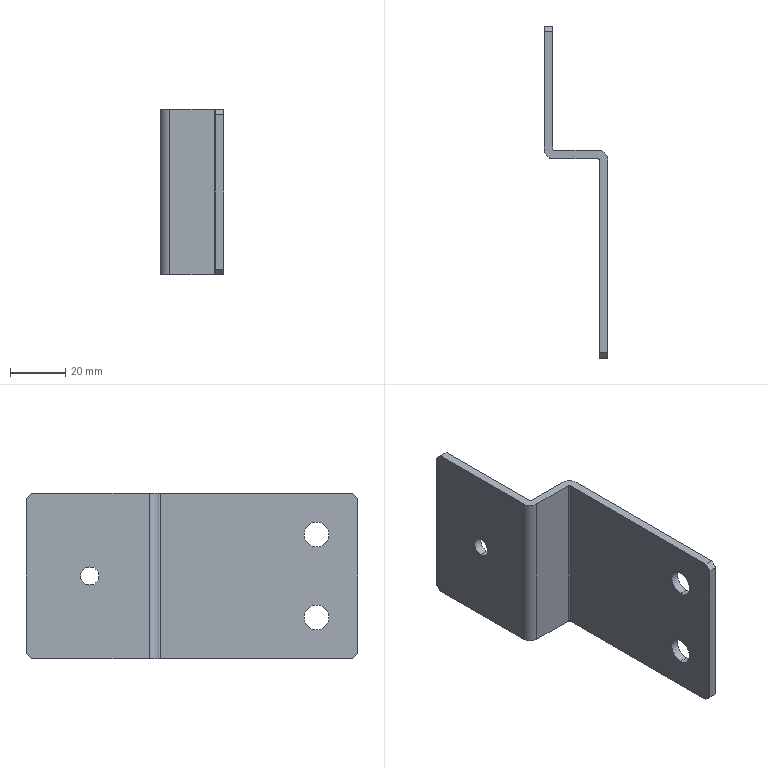Part | SolidWorks | features BaseBody 1 | 1 solid | 24 faces | box 23 x 120 x 60 mm | volume 24383 mm3 | plane 14 | cylinder 10 | commonest cylinder face diameters 9 x4 1 x2 6.6 x2 7 x2
STEP:
#1=CARTESIAN_POINT('',(17.,-60.,10.5));
#2=VERTEX_POINT('',#1);
#3=CARTESIAN_POINT('',(17.,-60.,19.5));
#4=VERTEX_POINT('',#3);
#5=CARTESIAN_POINT('',(17.,-60.,15.));
#6=DIRECTION('',(-1.,0.,0.));
#7=DIRECTION('',(0.,0.,-1.));
#8=AXIS2_PLACEMENT_3D('',#5,#6,#7);
#9=CIRCLE('',#8,4.5);
#10=EDGE_CURVE('',#2,#4,#9,.T.);
#11=ORIENTED_EDGE('',*,*,#10,.T.);
#12=CARTESIAN_POINT('',(20.,-60.,19.5));
#13=VERTEX_POINT('',#12);
#14=CARTESIAN_POINT('',(20.,-60.,19.5));
#15=DIRECTION('',(1.,0.,0.));
#16=VECTOR('',#15,1000.);
#17=LINE('',#14,#16);
#18=EDGE_CURVE('',#4,#13,#17,.T.);
#19=ORIENTED_EDGE('',*,*,#18,.T.);
#20=CARTESIAN_POINT('',(20.,-60.,10.5));
#21=VERTEX_POINT('',#20);
#22=CARTESIAN_POINT('',(20.,-60.,15.));
#23=DIRECTION('',(-1.,0.,0.));
#24=DIRECTION('',(0.,0.,-1.));
#25=AXIS2_PLACEMENT_3D('',#22,#23,#24);
#26=CIRCLE('',#25,4.5);
#27=EDGE_CURVE('',#21,#13,#26,.T.);
#28=ORIENTED_EDGE('',*,*,#27,.F.);
#29=CARTESIAN_POINT('',(20.,-60.,10.5));
#30=DIRECTION('',(1.,0.,0.));
#31=VECTOR('',#30,1000.);
#32=LINE('',#29,#31);
#33=EDGE_CURVE('',#2,#21,#32,.T.);
#34=ORIENTED_EDGE('',*,*,#33,.F.);
#35=EDGE_LOOP('',(#11,#19,#28,#34));
#36=FACE_OUTER_BOUND('',#35,.T.);
#37=CARTESIAN_POINT('',(20.,-60.,15.));
#38=DIRECTION('',(1.,0.,0.));
#39=DIRECTION('',(0.,0.,-1.));
#40=AXIS2_PLACEMENT_3D('',#37,#38,#39);
#41=CYLINDRICAL_SURFACE('',#40,4.5);
#42=ADVANCED_FACE('',(#36),#41,.F.);
#43=CARTESIAN_POINT('',(17.,-60.,40.5));
#44=VERTEX_POINT('',#43);
#45=CARTESIAN_POINT('',(17.,-60.,49.5));
#46=VERTEX_POINT('',#45);
#47=CARTESIAN_POINT('',(17.,-60.,45.));
#48=DIRECTION('',(-1.,0.,0.));
#49=DIRECTION('',(0.,0.,-1.));
#50=AXIS2_PLACEMENT_3D('',#47,#48,#49);
#51=CIRCLE('',#50,4.5);
#52=EDGE_CURVE('',#44,#46,#51,.T.);
#53=ORIENTED_EDGE('',*,*,#52,.T.);
#54=CARTESIAN_POINT('',(20.,-60.,49.5));
#55=VERTEX_POINT('',#54);
#56=CARTESIAN_POINT('',(20.,-60.,49.5));
#57=DIRECTION('',(1.,0.,0.));
#58=VECTOR('',#57,1000.);
#59=LINE('',#56,#58);
#60=EDGE_CURVE('',#46,#55,#59,.T.);
#61=ORIENTED_EDGE('',*,*,#60,.T.);
#62=CARTESIAN_POINT('',(20.,-60.,40.5));
#63=VERTEX_POINT('',#62);
#64=CARTESIAN_POINT('',(20.,-60.,45.));
#65=DIRECTION('',(-1.,0.,0.));
#66=DIRECTION('',(0.,0.,-1.));
#67=AXIS2_PLACEMENT_3D('',#64,#65,#66);
#68=CIRCLE('',#67,4.5);
#69=EDGE_CURVE('',#63,#55,#68,.T.);
#70=ORIENTED_EDGE('',*,*,#69,.F.);
#71=CARTESIAN_POINT('',(20.,-60.,40.5));
#72=DIRECTION('',(1.,0.,0.));
#73=VECTOR('',#72,1000.);
#74=LINE('',#71,#73);
#75=EDGE_CURVE('',#44,#63,#74,.T.);
#76=ORIENTED_EDGE('',*,*,#75,.F.);
#77=EDGE_LOOP('',(#53,#61,#70,#76));
#78=FACE_OUTER_BOUND('',#77,.T.);
#79=CARTESIAN_POINT('',(20.,-60.,45.));
#80=DIRECTION('',(1.,0.,0.));
#81=DIRECTION('',(0.,0.,-1.));
#82=AXIS2_PLACEMENT_3D('',#79,#80,#81);
#83=CYLINDRICAL_SURFACE('',#82,4.5);
#84=ADVANCED_FACE('',(#78),#83,.F.);
#85=CARTESIAN_POINT('',(-3.,22.,26.7));
#86=VERTEX_POINT('',#85);
#87=CARTESIAN_POINT('',(-3.,22.,33.3));
#88=VERTEX_POINT('',#87);
#89=CARTESIAN_POINT('',(-3.,22.,30.));
#90=DIRECTION('',(-1.,0.,0.));
#91=DIRECTION('',(0.,0.,-1.));
#92=AXIS2_PLACEMENT_3D('',#89,#90,#91);
#93=CIRCLE('',#92,3.3);
#94=EDGE_CURVE('',#86,#88,#93,.T.);
#95=ORIENTED_EDGE('',*,*,#94,.T.);
#96=CARTESIAN_POINT('',(0.,22.,33.3));
#97=VERTEX_POINT('',#96);
#98=CARTESIAN_POINT('',(0.,22.,33.3));
#99=DIRECTION('',(1.,0.,0.));
#100=VECTOR('',#99,1000.);
#101=LINE('',#98,#100);
#102=EDGE_CURVE('',#88,#97,#101,.T.);
#103=ORIENTED_EDGE('',*,*,#102,.T.);
#104=CARTESIAN_POINT('',(0.,22.,26.7));
#105=VERTEX_POINT('',#104);
#106=CARTESIAN_POINT('',(0.,22.,30.));
#107=DIRECTION('',(-1.,0.,0.));
#108=DIRECTION('',(0.,0.,-1.));
#109=AXIS2_PLACEMENT_3D('',#106,#107,#108);
#110=CIRCLE('',#109,3.3);
#111=EDGE_CURVE('',#105,#97,#110,.T.);
#112=ORIENTED_EDGE('',*,*,#111,.F.);
#113=CARTESIAN_POINT('',(0.,22.,26.7));
#114=DIRECTION('',(1.,0.,0.));
#115=VECTOR('',#114,1000.);
#116=LINE('',#113,#115);
#117=EDGE_CURVE('',#86,#105,#116,.T.);
#118=ORIENTED_EDGE('',*,*,#117,.F.);
#119=EDGE_LOOP('',(#95,#103,#112,#118));
#120=FACE_OUTER_BOUND('',#119,.T.);
#121=CARTESIAN_POINT('',(0.,22.,30.));
#122=DIRECTION('',(1.,0.,0.));
#123=DIRECTION('',(0.,0.,-1.));
#124=AXIS2_PLACEMENT_3D('',#121,#122,#123);
#125=CYLINDRICAL_SURFACE('',#124,3.3);
#126=ADVANCED_FACE('',(#120),#125,.F.);
#127=CARTESIAN_POINT('',(17.,-75.,2.));
#128=VERTEX_POINT('',#127);
#129=CARTESIAN_POINT('',(17.,-73.,0.));
#130=VERTEX_POINT('',#129);
#131=CARTESIAN_POINT('',(17.,-75.,2.));
#132=DIRECTION('',(0.,0.7071,-0.7071));
#133=VECTOR('',#132,1000.);
#134=LINE('',#131,#133);
#135=EDGE_CURVE('',#128,#130,#134,.T.);
#136=ORIENTED_EDGE('',*,*,#135,.F.);
#137=CARTESIAN_POINT('',(17.,-75.,58.));
#138=VERTEX_POINT('',#137);
#139=CARTESIAN_POINT('',(17.,-75.,60.));
#140=DIRECTION('',(0.,0.,-1.));
#141=VECTOR('',#140,1000.);
#142=LINE('',#139,#141);
#143=EDGE_CURVE('',#138,#128,#142,.T.);
#144=ORIENTED_EDGE('',*,*,#143,.F.);
#145=CARTESIAN_POINT('',(17.,-73.,60.));
#146=VERTEX_POINT('',#145);
#147=CARTESIAN_POINT('',(17.,-73.,60.));
#148=DIRECTION('',(0.,-0.7071,-0.7071));
#149=VECTOR('',#148,1000.);
#150=LINE('',#147,#149);
#151=EDGE_CURVE('',#146,#138,#150,.T.);
#152=ORIENTED_EDGE('',*,*,#151,.F.);
#153=CARTESIAN_POINT('',(17.,-3.5,60.));
#154=VERTEX_POINT('',#153);
#155=CARTESIAN_POINT('',(17.,0.,60.));
#156=DIRECTION('',(0.,-1.,0.));
#157=VECTOR('',#156,1000.);
#158=LINE('',#155,#157);
#159=EDGE_CURVE('',#154,#146,#158,.T.);
#160=ORIENTED_EDGE('',*,*,#159,.F.);
#161=CARTESIAN_POINT('',(17.,-3.5,0.));
#162=VERTEX_POINT('',#161);
#163=CARTESIAN_POINT('',(17.,-3.5,60.));
#164=DIRECTION('',(0.,0.,1.));
#165=VECTOR('',#164,1000.);
#166=LINE('',#163,#165);
#167=EDGE_CURVE('',#162,#154,#166,.T.);
#168=ORIENTED_EDGE('',*,*,#167,.F.);
#169=CARTESIAN_POINT('',(17.,0.,0.));
#170=DIRECTION('',(0.,1.,0.));
#171=VECTOR('',#170,1000.);
#172=LINE('',#169,#171);
#173=EDGE_CURVE('',#130,#162,#172,.T.);
#174=ORIENTED_EDGE('',*,*,#173,.F.);
#175=EDGE_LOOP('',(#136,#144,#152,#160,#168,#174));
#176=FACE_OUTER_BOUND('',#175,.T.);
#177=ORIENTED_EDGE('',*,*,#10,.F.);
#178=CARTESIAN_POINT('',(17.,-60.,15.));
#179=DIRECTION('',(-1.,0.,0.));
#180=DIRECTION('',(0.,0.,-1.));
#181=AXIS2_PLACEMENT_3D('',#178,#179,#180);
#182=CIRCLE('',#181,4.5);
#183=EDGE_CURVE('',#4,#2,#182,.T.);
#184=ORIENTED_EDGE('',*,*,#183,.F.);
#185=EDGE_LOOP('',(#177,#184));
#186=FACE_BOUND('',#185,.T.);
#187=ORIENTED_EDGE('',*,*,#52,.F.);
#188=CARTESIAN_POINT('',(17.,-60.,45.));
#189=DIRECTION('',(-1.,0.,0.));
#190=DIRECTION('',(0.,0.,-1.));
#191=AXIS2_PLACEMENT_3D('',#188,#189,#190);
#192=CIRCLE('',#191,4.5);
#193=EDGE_CURVE('',#46,#44,#192,.T.);
#194=ORIENTED_EDGE('',*,*,#193,.F.);
#195=EDGE_LOOP('',(#187,#194));
#196=FACE_BOUND('',#195,.T.);
#197=CARTESIAN_POINT('',(17.,0.,60.));
#198=DIRECTION('',(1.,0.,0.));
#199=DIRECTION('',(0.,1.,0.));
#200=AXIS2_PLACEMENT_3D('',#197,#198,#199);
#201=PLANE('',#200);
#202=ADVANCED_FACE('',(#176,#186,#196),#201,.F.);
#203=CARTESIAN_POINT('',(20.,-73.,0.));
#204=VERTEX_POINT('',#203);
#205=CARTESIAN_POINT('',(16.5,-73.,0.));
#206=DIRECTION('',(1.,0.,0.));
#207=VECTOR('',#206,1000.);
#208=LINE('',#205,#207);
#209=EDGE_CURVE('',#130,#204,#208,.T.);
#210=ORIENTED_EDGE('',*,*,#209,.F.);
#211=ORIENTED_EDGE('',*,*,#173,.T.);
#212=CARTESIAN_POINT('',(16.5,-3.,0.));
#213=VERTEX_POINT('',#212);
#214=CARTESIAN_POINT('',(16.5,-3.5,0.));
#215=DIRECTION('',(0.,0.,1.));
#216=DIRECTION('',(-1.,0.,0.));
#217=AXIS2_PLACEMENT_3D('',#214,#215,#216);
#218=CIRCLE('',#217,0.5);
#219=EDGE_CURVE('',#162,#213,#218,.T.);
#220=ORIENTED_EDGE('',*,*,#219,.T.);
#221=CARTESIAN_POINT('',(0.5,-3.,0.));
#222=VERTEX_POINT('',#221);
#223=CARTESIAN_POINT('',(0.,-3.,0.));
#224=DIRECTION('',(-1.,0.,0.));
#225=VECTOR('',#224,1000.);
#226=LINE('',#223,#225);
#227=EDGE_CURVE('',#213,#222,#226,.T.);
#228=ORIENTED_EDGE('',*,*,#227,.T.);
#229=CARTESIAN_POINT('',(-3.,0.5,0.));
#230=VERTEX_POINT('',#229);
#231=CARTESIAN_POINT('',(0.5,0.5,0.));
#232=DIRECTION('',(0.,0.,1.));
#233=DIRECTION('',(-1.,0.,0.));
#234=AXIS2_PLACEMENT_3D('',#231,#232,#233);
#235=CIRCLE('',#234,3.5);
#236=EDGE_CURVE('',#230,#222,#235,.T.);
#237=ORIENTED_EDGE('',*,*,#236,.F.);
#238=CARTESIAN_POINT('',(-3.,43.,0.));
#239=VERTEX_POINT('',#238);
#240=CARTESIAN_POINT('',(-3.,45.,0.));
#241=DIRECTION('',(0.,1.,0.));
#242=VECTOR('',#241,1000.);
#243=LINE('',#240,#242);
#244=EDGE_CURVE('',#230,#239,#243,.T.);
#245=ORIENTED_EDGE('',*,*,#244,.T.);
#246=CARTESIAN_POINT('',(0.,43.,0.));
#247=VERTEX_POINT('',#246);
#248=CARTESIAN_POINT('',(0.5,43.,0.));
#249=DIRECTION('',(1.,0.,0.));
#250=VECTOR('',#249,1000.);
#251=LINE('',#248,#250);
#252=EDGE_CURVE('',#239,#247,#251,.T.);
#253=ORIENTED_EDGE('',*,*,#252,.T.);
#254=CARTESIAN_POINT('',(0.,0.5,0.));
#255=VERTEX_POINT('',#254);
#256=CARTESIAN_POINT('',(0.,-3.,0.));
#257=DIRECTION('',(0.,-1.,0.));
#258=VECTOR('',#257,1000.);
#259=LINE('',#256,#258);
#260=EDGE_CURVE('',#247,#255,#259,.T.);
#261=ORIENTED_EDGE('',*,*,#260,.T.);
#262=CARTESIAN_POINT('',(0.5,0.,0.));
#263=VERTEX_POINT('',#262);
#264=CARTESIAN_POINT('',(0.5,0.5,0.));
#265=DIRECTION('',(0.,0.,1.));
#266=DIRECTION('',(-1.,0.,0.));
#267=AXIS2_PLACEMENT_3D('',#264,#265,#266);
#268=CIRCLE('',#267,0.5);
#269=EDGE_CURVE('',#255,#263,#268,.T.);
#270=ORIENTED_EDGE('',*,*,#269,.T.);
#271=CARTESIAN_POINT('',(16.5,0.,0.));
#272=VERTEX_POINT('',#271);
#273=CARTESIAN_POINT('',(17.,0.,0.));
#274=DIRECTION('',(1.,0.,0.));
#275=VECTOR('',#274,1000.);
#276=LINE('',#273,#275);
#277=EDGE_CURVE('',#263,#272,#276,.T.);
#278=ORIENTED_EDGE('',*,*,#277,.T.);
#279=CARTESIAN_POINT('',(20.,-3.5,0.));
#280=VERTEX_POINT('',#279);
#281=CARTESIAN_POINT('',(16.5,-3.5,0.));
#282=DIRECTION('',(0.,0.,-1.));
#283=DIRECTION('',(-1.,0.,0.));
#284=AXIS2_PLACEMENT_3D('',#281,#282,#283);
#285=CIRCLE('',#284,3.5);
#286=EDGE_CURVE('',#272,#280,#285,.T.);
#287=ORIENTED_EDGE('',*,*,#286,.T.);
#288=CARTESIAN_POINT('',(20.,-3.5,0.));
#289=DIRECTION('',(0.,1.,0.));
#290=VECTOR('',#289,1000.);
#291=LINE('',#288,#290);
#292=EDGE_CURVE('',#204,#280,#291,.T.);
#293=ORIENTED_EDGE('',*,*,#292,.F.);
#294=EDGE_LOOP('',(#210,#211,#220,#228,#237,#245,#253,#261,#270,#278,#287,#293));
#295=FACE_OUTER_BOUND('',#294,.T.);
#296=CARTESIAN_POINT('',(16.5,-3.5,0.));
#297=DIRECTION('',(0.,0.,1.));
#298=DIRECTION('',(1.,0.,0.));
#299=AXIS2_PLACEMENT_3D('',#296,#297,#298);
#300=PLANE('',#299);
#301=ADVANCED_FACE('',(#295),#300,.F.);
#302=ORIENTED_EDGE('',*,*,#135,.T.);
#303=ORIENTED_EDGE('',*,*,#209,.T.);
#304=CARTESIAN_POINT('',(20.,-75.,2.));
#305=VERTEX_POINT('',#304);
#306=CARTESIAN_POINT('',(20.,-73.,0.));
#307=DIRECTION('',(0.,-0.7071,0.7071));
#308=VECTOR('',#307,1000.);
#309=LINE('',#306,#308);
#310=EDGE_CURVE('',#204,#305,#309,.T.);
#311=ORIENTED_EDGE('',*,*,#310,.T.);
#312=CARTESIAN_POINT('',(16.5,-75.,2.));
#313=DIRECTION('',(-1.,0.,0.));
#314=VECTOR('',#313,1000.);
#315=LINE('',#312,#314);
#316=EDGE_CURVE('',#305,#128,#315,.T.);
#317=ORIENTED_EDGE('',*,*,#316,.T.);
#318=EDGE_LOOP('',(#302,#303,#311,#317));
#319=FACE_OUTER_BOUND('',#318,.T.);
#320=CARTESIAN_POINT('',(16.5,-73.,0.));
#321=DIRECTION('',(0.,-0.7071,-0.7071));
#322=DIRECTION('',(0.,0.7071,-0.7071));
#323=AXIS2_PLACEMENT_3D('',#320,#321,#322);
#324=PLANE('',#323);
#325=ADVANCED_FACE('',(#319),#324,.T.);
#326=CARTESIAN_POINT('',(20.,-75.,58.));
#327=VERTEX_POINT('',#326);
#328=CARTESIAN_POINT('',(20.,-75.,60.));
#329=DIRECTION('',(0.,0.,1.));
#330=VECTOR('',#329,1000.);
#331=LINE('',#328,#330);
#332=EDGE_CURVE('',#305,#327,#331,.T.);
#333=ORIENTED_EDGE('',*,*,#332,.T.);
#334=CARTESIAN_POINT('',(20.,-75.,58.));
#335=DIRECTION('',(-1.,0.,0.));
#336=VECTOR('',#335,1000.);
#337=LINE('',#334,#336);
#338=EDGE_CURVE('',#327,#138,#337,.T.);
#339=ORIENTED_EDGE('',*,*,#338,.T.);
#340=ORIENTED_EDGE('',*,*,#143,.T.);
#341=ORIENTED_EDGE('',*,*,#316,.F.);
#342=EDGE_LOOP('',(#333,#339,#340,#341));
#343=FACE_OUTER_BOUND('',#342,.T.);
#344=CARTESIAN_POINT('',(20.,-75.,60.));
#345=DIRECTION('',(0.,-1.,0.));
#346=DIRECTION('',(0.,0.,-1.));
#347=AXIS2_PLACEMENT_3D('',#344,#345,#346);
#348=PLANE('',#347);
#349=ADVANCED_FACE('',(#343),#348,.T.);
#350=CARTESIAN_POINT('',(20.,-73.,60.));
#351=VERTEX_POINT('',#350);
#352=CARTESIAN_POINT('',(20.,-73.,60.));
#353=DIRECTION('',(1.,0.,0.));
#354=VECTOR('',#353,1000.);
#355=LINE('',#352,#354);
#356=EDGE_CURVE('',#146,#351,#355,.T.);
#357=ORIENTED_EDGE('',*,*,#356,.F.);
#358=ORIENTED_EDGE('',*,*,#151,.T.);
#359=ORIENTED_EDGE('',*,*,#338,.F.);
#360=CARTESIAN_POINT('',(20.,-75.,58.));
#361=DIRECTION('',(0.,-0.7071,-0.7071));
#362=VECTOR('',#361,1000.);
#363=LINE('',#360,#362);
#364=EDGE_CURVE('',#351,#327,#363,.T.);
#365=ORIENTED_EDGE('',*,*,#364,.F.);
#366=EDGE_LOOP('',(#357,#358,#359,#365));
#367=FACE_OUTER_BOUND('',#366,.T.);
#368=CARTESIAN_POINT('',(20.,-75.,58.));
#369=DIRECTION('',(0.,0.7071,-0.7071));
#370=DIRECTION('',(0.,0.7071,0.7071));
#371=AXIS2_PLACEMENT_3D('',#368,#369,#370);
#372=PLANE('',#371);
#373=ADVANCED_FACE('',(#367),#372,.F.);
#374=CARTESIAN_POINT('',(20.,-3.5,60.));
#375=VERTEX_POINT('',#374);
#376=CARTESIAN_POINT('',(20.,-3.,60.));
#377=DIRECTION('',(0.,1.,0.));
#378=VECTOR('',#377,1000.);
#379=LINE('',#376,#378);
#380=EDGE_CURVE('',#351,#375,#379,.T.);
#381=ORIENTED_EDGE('',*,*,#380,.T.);
#382=CARTESIAN_POINT('',(16.5,0.,60.));
#383=VERTEX_POINT('',#382);
#384=CARTESIAN_POINT('',(16.5,-3.5,60.));
#385=DIRECTION('',(0.,0.,1.));
#386=DIRECTION('',(-1.,0.,0.));
#387=AXIS2_PLACEMENT_3D('',#384,#385,#386);
#388=CIRCLE('',#387,3.5);
#389=EDGE_CURVE('',#375,#383,#388,.T.);
#390=ORIENTED_EDGE('',*,*,#389,.T.);
#391=CARTESIAN_POINT('',(0.5,0.,60.));
#392=VERTEX_POINT('',#391);
#393=CARTESIAN_POINT('',(-3.,0.,60.));
#394=DIRECTION('',(-1.,0.,0.));
#395=VECTOR('',#394,1000.);
#396=LINE('',#393,#395);
#397=EDGE_CURVE('',#383,#392,#396,.T.);
#398=ORIENTED_EDGE('',*,*,#397,.T.);
#399=CARTESIAN_POINT('',(0.,0.5,60.));
#400=VERTEX_POINT('',#399);
#401=CARTESIAN_POINT('',(0.5,0.5,60.));
#402=DIRECTION('',(0.,0.,-1.));
#403=DIRECTION('',(-1.,0.,0.));
#404=AXIS2_PLACEMENT_3D('',#401,#402,#403);
#405=CIRCLE('',#404,0.5);
#406=EDGE_CURVE('',#392,#400,#405,.T.);
#407=ORIENTED_EDGE('',*,*,#406,.T.);
#408=CARTESIAN_POINT('',(0.,43.,60.));
#409=VERTEX_POINT('',#408);
#410=CARTESIAN_POINT('',(0.,-3.5,60.));
#411=DIRECTION('',(0.,1.,0.));
#412=VECTOR('',#411,1000.);
#413=LINE('',#410,#412);
#414=EDGE_CURVE('',#400,#409,#413,.T.);
#415=ORIENTED_EDGE('',*,*,#414,.T.);
#416=CARTESIAN_POINT('',(-3.,43.,60.));
#417=VERTEX_POINT('',#416);
#418=CARTESIAN_POINT('',(16.5,43.,60.));
#419=DIRECTION('',(-1.,0.,0.));
#420=VECTOR('',#419,1000.);
#421=LINE('',#418,#420);
#422=EDGE_CURVE('',#409,#417,#421,.T.);
#423=ORIENTED_EDGE('',*,*,#422,.T.);
#424=CARTESIAN_POINT('',(-3.,0.5,60.));
#425=VERTEX_POINT('',#424);
#426=CARTESIAN_POINT('',(-3.,45.,60.));
#427=DIRECTION('',(0.,-1.,0.));
#428=VECTOR('',#427,1000.);
#429=LINE('',#426,#428);
#430=EDGE_CURVE('',#417,#425,#429,.T.);
#431=ORIENTED_EDGE('',*,*,#430,.T.);
#432=CARTESIAN_POINT('',(0.5,-3.,60.));
#433=VERTEX_POINT('',#432);
#434=CARTESIAN_POINT('',(0.5,0.5,60.));
#435=DIRECTION('',(0.,0.,-1.));
#436=DIRECTION('',(-1.,0.,0.));
#437=AXIS2_PLACEMENT_3D('',#434,#435,#436);
#438=CIRCLE('',#437,3.5);
#439=EDGE_CURVE('',#433,#425,#438,.T.);
#440=ORIENTED_EDGE('',*,*,#439,.F.);
#441=CARTESIAN_POINT('',(16.5,-3.,60.));
#442=VERTEX_POINT('',#441);
#443=CARTESIAN_POINT('',(0.,-3.,60.));
#444=DIRECTION('',(1.,0.,0.));
#445=VECTOR('',#444,1000.);
#446=LINE('',#443,#445);
#447=EDGE_CURVE('',#433,#442,#446,.T.);
#448=ORIENTED_EDGE('',*,*,#447,.T.);
#449=CARTESIAN_POINT('',(16.5,-3.5,60.));
#450=DIRECTION('',(0.,0.,-1.));
#451=DIRECTION('',(-1.,0.,0.));
#452=AXIS2_PLACEMENT_3D('',#449,#450,#451);
#453=CIRCLE('',#452,0.5);
#454=EDGE_CURVE('',#442,#154,#453,.T.);
#455=ORIENTED_EDGE('',*,*,#454,.T.);
#456=ORIENTED_EDGE('',*,*,#159,.T.);
#457=ORIENTED_EDGE('',*,*,#356,.T.);
#458=EDGE_LOOP('',(#381,#390,#398,#407,#415,#423,#431,#440,#448,#455,#456,#457));
#459=FACE_OUTER_BOUND('',#458,.T.);
#460=CARTESIAN_POINT('',(16.5,-3.,60.));
#461=DIRECTION('',(0.,0.,1.));
#462=DIRECTION('',(1.,0.,0.));
#463=AXIS2_PLACEMENT_3D('',#460,#461,#462);
#464=PLANE('',#463);
#465=ADVANCED_FACE('',(#459),#464,.T.);
#466=ORIENTED_EDGE('',*,*,#167,.T.);
#467=ORIENTED_EDGE('',*,*,#454,.F.);
#468=CARTESIAN_POINT('',(16.5,-3.,60.));
#469=DIRECTION('',(0.,0.,1.));
#470=VECTOR('',#469,1000.);
#471=LINE('',#468,#470);
#472=EDGE_CURVE('',#213,#442,#471,.T.);
#473=ORIENTED_EDGE('',*,*,#472,.F.);
#474=ORIENTED_EDGE('',*,*,#219,.F.);
#475=EDGE_LOOP('',(#466,#467,#473,#474));
#476=FACE_OUTER_BOUND('',#475,.T.);
#477=CARTESIAN_POINT('',(16.5,-3.5,60.));
#478=DIRECTION('',(0.,0.,-1.));
#479=DIRECTION('',(-1.,0.,0.));
#480=AXIS2_PLACEMENT_3D('',#477,#478,#479);
#481=CYLINDRICAL_SURFACE('',#480,0.5);
#482=ADVANCED_FACE('',(#476),#481,.F.);
#483=ORIENTED_EDGE('',*,*,#18,.F.);
#484=ORIENTED_EDGE('',*,*,#183,.T.);
#485=ORIENTED_EDGE('',*,*,#33,.T.);
#486=CARTESIAN_POINT('',(20.,-60.,15.));
#487=DIRECTION('',(-1.,0.,0.));
#488=DIRECTION('',(0.,0.,-1.));
#489=AXIS2_PLACEMENT_3D('',#486,#487,#488);
#490=CIRCLE('',#489,4.5);
#491=EDGE_CURVE('',#13,#21,#490,.T.);
#492=ORIENTED_EDGE('',*,*,#491,.F.);
#493=EDGE_LOOP('',(#483,#484,#485,#492));
#494=FACE_OUTER_BOUND('',#493,.T.);
#495=CARTESIAN_POINT('',(20.,-60.,15.));
#496=DIRECTION('',(1.,0.,0.));
#497=DIRECTION('',(0.,0.,-1.));
#498=AXIS2_PLACEMENT_3D('',#495,#496,#497);
#499=CYLINDRICAL_SURFACE('',#498,4.5);
#500=ADVANCED_FACE('',(#494),#499,.F.);
#501=ORIENTED_EDGE('',*,*,#60,.F.);
#502=ORIENTED_EDGE('',*,*,#193,.T.);
#503=ORIENTED_EDGE('',*,*,#75,.T.);
#504=CARTESIAN_POINT('',(20.,-60.,45.));
#505=DIRECTION('',(-1.,0.,0.));
#506=DIRECTION('',(0.,0.,-1.));
#507=AXIS2_PLACEMENT_3D('',#504,#505,#506);
#508=CIRCLE('',#507,4.5);
#509=EDGE_CURVE('',#55,#63,#508,.T.);
#510=ORIENTED_EDGE('',*,*,#509,.F.);
#511=EDGE_LOOP('',(#501,#502,#503,#510));
#512=FACE_OUTER_BOUND('',#511,.T.);
#513=CARTESIAN_POINT('',(20.,-60.,45.));
#514=DIRECTION('',(1.,0.,0.));
#515=DIRECTION('',(0.,0.,-1.));
#516=AXIS2_PLACEMENT_3D('',#513,#514,#515);
#517=CYLINDRICAL_SURFACE('',#516,4.5);
#518=ADVANCED_FACE('',(#512),#517,.F.);
#519=ORIENTED_EDGE('',*,*,#380,.F.);
#520=ORIENTED_EDGE('',*,*,#364,.T.);
#521=ORIENTED_EDGE('',*,*,#332,.F.);
#522=ORIENTED_EDGE('',*,*,#310,.F.);
#523=ORIENTED_EDGE('',*,*,#292,.T.);
#524=CARTESIAN_POINT('',(20.,-3.5,60.));
#525=DIRECTION('',(0.,0.,1.));
#526=VECTOR('',#525,1000.);
#527=LINE('',#524,#526);
#528=EDGE_CURVE('',#280,#375,#527,.T.);
#529=ORIENTED_EDGE('',*,*,#528,.T.);
#530=EDGE_LOOP('',(#519,#520,#521,#522,#523,#529));
#531=FACE_OUTER_BOUND('',#530,.T.);
#532=ORIENTED_EDGE('',*,*,#27,.T.);
#533=ORIENTED_EDGE('',*,*,#491,.T.);
#534=EDGE_LOOP('',(#532,#533));
#535=FACE_BOUND('',#534,.T.);
#536=ORIENTED_EDGE('',*,*,#69,.T.);
#537=ORIENTED_EDGE('',*,*,#509,.T.);
#538=EDGE_LOOP('',(#536,#537));
#539=FACE_BOUND('',#538,.T.);
#540=CARTESIAN_POINT('',(20.,0.,60.));
#541=DIRECTION('',(1.,0.,0.));
#542=DIRECTION('',(0.,1.,0.));
#543=AXIS2_PLACEMENT_3D('',#540,#541,#542);
#544=PLANE('',#543);
#545=ADVANCED_FACE('',(#531,#535,#539),#544,.T.);
#546=ORIENTED_EDGE('',*,*,#472,.T.);
#547=ORIENTED_EDGE('',*,*,#447,.F.);
#548=CARTESIAN_POINT('',(0.5,-3.,60.));
#549=DIRECTION('',(0.,0.,1.));
#550=VECTOR('',#549,1000.);
#551=LINE('',#548,#550);
#552=EDGE_CURVE('',#222,#433,#551,.T.);
#553=ORIENTED_EDGE('',*,*,#552,.F.);
#554=ORIENTED_EDGE('',*,*,#227,.F.);
#555=EDGE_LOOP('',(#546,#547,#553,#554));
#556=FACE_OUTER_BOUND('',#555,.T.);
#557=CARTESIAN_POINT('',(0.,-3.,60.));
#558=DIRECTION('',(0.,1.,0.));
#559=DIRECTION('',(0.,0.,1.));
#560=AXIS2_PLACEMENT_3D('',#557,#558,#559);
#561=PLANE('',#560);
#562=ADVANCED_FACE('',(#556),#561,.F.);
#563=ORIENTED_EDGE('',*,*,#389,.F.);
#564=ORIENTED_EDGE('',*,*,#528,.F.);
#565=ORIENTED_EDGE('',*,*,#286,.F.);
#566=CARTESIAN_POINT('',(16.5,0.,60.));
#567=DIRECTION('',(0.,0.,1.));
#568=VECTOR('',#567,1000.);
#569=LINE('',#566,#568);
#570=EDGE_CURVE('',#272,#383,#569,.T.);
#571=ORIENTED_EDGE('',*,*,#570,.T.);
#572=EDGE_LOOP('',(#563,#564,#565,#571));
#573=FACE_OUTER_BOUND('',#572,.T.);
#574=CARTESIAN_POINT('',(16.5,-3.5,60.));
#575=DIRECTION('',(0.,0.,-1.));
#576=DIRECTION('',(-1.,0.,0.));
#577=AXIS2_PLACEMENT_3D('',#574,#575,#576);
#578=CYLINDRICAL_SURFACE('',#577,3.5);
#579=ADVANCED_FACE('',(#573),#578,.T.);
#580=ORIENTED_EDGE('',*,*,#439,.T.);
#581=CARTESIAN_POINT('',(-3.,0.5,60.));
#582=DIRECTION('',(0.,0.,-1.));
#583=VECTOR('',#582,1000.);
#584=LINE('',#581,#583);
#585=EDGE_CURVE('',#425,#230,#584,.T.);
#586=ORIENTED_EDGE('',*,*,#585,.T.);
#587=ORIENTED_EDGE('',*,*,#236,.T.);
#588=ORIENTED_EDGE('',*,*,#552,.T.);
#589=EDGE_LOOP('',(#580,#586,#587,#588));
#590=FACE_OUTER_BOUND('',#589,.T.);
#591=CARTESIAN_POINT('',(0.5,0.5,60.));
#592=DIRECTION('',(0.,0.,-1.));
#593=DIRECTION('',(-1.,0.,0.));
#594=AXIS2_PLACEMENT_3D('',#591,#592,#593);
#595=CYLINDRICAL_SURFACE('',#594,3.5);
#596=ADVANCED_FACE('',(#590),#595,.T.);
#597=ORIENTED_EDGE('',*,*,#397,.F.);
#598=ORIENTED_EDGE('',*,*,#570,.F.);
#599=ORIENTED_EDGE('',*,*,#277,.F.);
#600=CARTESIAN_POINT('',(0.5,0.,60.));
#601=DIRECTION('',(0.,0.,1.));
#602=VECTOR('',#601,1000.);
#603=LINE('',#600,#602);
#604=EDGE_CURVE('',#263,#392,#603,.T.);
#605=ORIENTED_EDGE('',*,*,#604,.T.);
#606=EDGE_LOOP('',(#597,#598,#599,#605));
#607=FACE_OUTER_BOUND('',#606,.T.);
#608=CARTESIAN_POINT('',(0.,0.,60.));
#609=DIRECTION('',(0.,1.,0.));
#610=DIRECTION('',(0.,0.,1.));
#611=AXIS2_PLACEMENT_3D('',#608,#609,#610);
#612=PLANE('',#611);
#613=ADVANCED_FACE('',(#607),#612,.T.);
#614=CARTESIAN_POINT('',(-3.,45.,58.));
#615=VERTEX_POINT('',#614);
#616=CARTESIAN_POINT('',(-3.,45.,58.));
#617=DIRECTION('',(0.,-0.7071,0.7071));
#618=VECTOR('',#617,1000.);
#619=LINE('',#616,#618);
#620=EDGE_CURVE('',#615,#417,#619,.T.);
#621=ORIENTED_EDGE('',*,*,#620,.F.);
#622=CARTESIAN_POINT('',(-3.,45.,2.));
#623=VERTEX_POINT('',#622);
#624=CARTESIAN_POINT('',(-3.,45.,60.));
#625=DIRECTION('',(0.,0.,1.));
#626=VECTOR('',#625,1000.);
#627=LINE('',#624,#626);
#628=EDGE_CURVE('',#623,#615,#627,.T.);
#629=ORIENTED_EDGE('',*,*,#628,.F.);
#630=CARTESIAN_POINT('',(-3.,43.,0.));
#631=DIRECTION('',(0.,0.7071,0.7071));
#632=VECTOR('',#631,1000.);
#633=LINE('',#630,#632);
#634=EDGE_CURVE('',#239,#623,#633,.T.);
#635=ORIENTED_EDGE('',*,*,#634,.F.);
#636=ORIENTED_EDGE('',*,*,#244,.F.);
#637=ORIENTED_EDGE('',*,*,#585,.F.);
#638=ORIENTED_EDGE('',*,*,#430,.F.);
#639=EDGE_LOOP('',(#621,#629,#635,#636,#637,#638));
#640=FACE_OUTER_BOUND('',#639,.T.);
#641=ORIENTED_EDGE('',*,*,#94,.F.);
#642=CARTESIAN_POINT('',(-3.,22.,30.));
#643=DIRECTION('',(-1.,0.,0.));
#644=DIRECTION('',(0.,0.,-1.));
#645=AXIS2_PLACEMENT_3D('',#642,#643,#644);
#646=CIRCLE('',#645,3.3);
#647=EDGE_CURVE('',#88,#86,#646,.T.);
#648=ORIENTED_EDGE('',*,*,#647,.F.);
#649=EDGE_LOOP('',(#641,#648));
#650=FACE_BOUND('',#649,.T.);
#651=CARTESIAN_POINT('',(-3.,45.,60.));
#652=DIRECTION('',(1.,0.,0.));
#653=DIRECTION('',(0.,1.,0.));
#654=AXIS2_PLACEMENT_3D('',#651,#652,#653);
#655=PLANE('',#654);
#656=ADVANCED_FACE('',(#640,#650),#655,.F.);
#657=CARTESIAN_POINT('',(0.,0.5,60.));
#658=DIRECTION('',(0.,0.,-1.));
#659=VECTOR('',#658,1000.);
#660=LINE('',#657,#659);
#661=EDGE_CURVE('',#400,#255,#660,.T.);
#662=ORIENTED_EDGE('',*,*,#661,.F.);
#663=ORIENTED_EDGE('',*,*,#406,.F.);
#664=ORIENTED_EDGE('',*,*,#604,.F.);
#665=ORIENTED_EDGE('',*,*,#269,.F.);
#666=EDGE_LOOP('',(#662,#663,#664,#665));
#667=FACE_OUTER_BOUND('',#666,.T.);
#668=CARTESIAN_POINT('',(0.5,0.5,60.));
#669=DIRECTION('',(0.,0.,-1.));
#670=DIRECTION('',(-1.,0.,0.));
#671=AXIS2_PLACEMENT_3D('',#668,#669,#670);
#672=CYLINDRICAL_SURFACE('',#671,0.5);
#673=ADVANCED_FACE('',(#667),#672,.F.);
#674=ORIENTED_EDGE('',*,*,#422,.F.);
#675=CARTESIAN_POINT('',(0.,45.,58.));
#676=VERTEX_POINT('',#675);
#677=CARTESIAN_POINT('',(0.,45.,58.));
#678=DIRECTION('',(0.,-0.7071,0.7071));
#679=VECTOR('',#678,1000.);
#680=LINE('',#677,#679);
#681=EDGE_CURVE('',#676,#409,#680,.T.);
#682=ORIENTED_EDGE('',*,*,#681,.F.);
#683=CARTESIAN_POINT('',(-3.,45.,58.));
#684=DIRECTION('',(1.,0.,0.));
#685=VECTOR('',#684,1000.);
#686=LINE('',#683,#685);
#687=EDGE_CURVE('',#615,#676,#686,.T.);
#688=ORIENTED_EDGE('',*,*,#687,.F.);
#689=ORIENTED_EDGE('',*,*,#620,.T.);
#690=EDGE_LOOP('',(#674,#682,#688,#689));
#691=FACE_OUTER_BOUND('',#690,.T.);
#692=CARTESIAN_POINT('',(-3.,45.,58.));
#693=DIRECTION('',(0.,-0.7071,-0.7071));
#694=DIRECTION('',(0.,0.7071,-0.7071));
#695=AXIS2_PLACEMENT_3D('',#692,#693,#694);
#696=PLANE('',#695);
#697=ADVANCED_FACE('',(#691),#696,.F.);
#698=CARTESIAN_POINT('',(0.,45.,2.));
#699=VERTEX_POINT('',#698);
#700=CARTESIAN_POINT('',(0.,45.,60.));
#701=DIRECTION('',(0.,0.,-1.));
#702=VECTOR('',#701,1000.);
#703=LINE('',#700,#702);
#704=EDGE_CURVE('',#676,#699,#703,.T.);
#705=ORIENTED_EDGE('',*,*,#704,.T.);
#706=CARTESIAN_POINT('',(-3.,45.,2.));
#707=DIRECTION('',(-1.,0.,0.));
#708=VECTOR('',#707,1000.);
#709=LINE('',#706,#708);
#710=EDGE_CURVE('',#699,#623,#709,.T.);
#711=ORIENTED_EDGE('',*,*,#710,.T.);
#712=ORIENTED_EDGE('',*,*,#628,.T.);
#713=ORIENTED_EDGE('',*,*,#687,.T.);
#714=EDGE_LOOP('',(#705,#711,#712,#713));
#715=FACE_OUTER_BOUND('',#714,.T.);
#716=CARTESIAN_POINT('',(-3.,45.,60.));
#717=DIRECTION('',(0.,1.,0.));
#718=DIRECTION('',(0.,0.,1.));
#719=AXIS2_PLACEMENT_3D('',#716,#717,#718);
#720=PLANE('',#719);
#721=ADVANCED_FACE('',(#715),#720,.T.);
#722=ORIENTED_EDGE('',*,*,#710,.F.);
#723=CARTESIAN_POINT('',(0.,43.,0.));
#724=DIRECTION('',(0.,0.7071,0.7071));
#725=VECTOR('',#724,1000.);
#726=LINE('',#723,#725);
#727=EDGE_CURVE('',#247,#699,#726,.T.);
#728=ORIENTED_EDGE('',*,*,#727,.F.);
#729=ORIENTED_EDGE('',*,*,#252,.F.);
#730=ORIENTED_EDGE('',*,*,#634,.T.);
#731=EDGE_LOOP('',(#722,#728,#729,#730));
#732=FACE_OUTER_BOUND('',#731,.T.);
#733=CARTESIAN_POINT('',(0.5,43.,0.));
#734=DIRECTION('',(0.,-0.7071,0.7071));
#735=DIRECTION('',(0.,-0.7071,-0.7071));
#736=AXIS2_PLACEMENT_3D('',#733,#734,#735);
#737=PLANE('',#736);
#738=ADVANCED_FACE('',(#732),#737,.F.);
#739=ORIENTED_EDGE('',*,*,#102,.F.);
#740=ORIENTED_EDGE('',*,*,#647,.T.);
#741=ORIENTED_EDGE('',*,*,#117,.T.);
#742=CARTESIAN_POINT('',(0.,22.,30.));
#743=DIRECTION('',(-1.,0.,0.));
#744=DIRECTION('',(0.,0.,-1.));
#745=AXIS2_PLACEMENT_3D('',#742,#743,#744);
#746=CIRCLE('',#745,3.3);
#747=EDGE_CURVE('',#97,#105,#746,.T.);
#748=ORIENTED_EDGE('',*,*,#747,.F.);
#749=EDGE_LOOP('',(#739,#740,#741,#748));
#750=FACE_OUTER_BOUND('',#749,.T.);
#751=CARTESIAN_POINT('',(0.,22.,30.));
#752=DIRECTION('',(1.,0.,0.));
#753=DIRECTION('',(0.,0.,-1.));
#754=AXIS2_PLACEMENT_3D('',#751,#752,#753);
#755=CYLINDRICAL_SURFACE('',#754,3.3);
#756=ADVANCED_FACE('',(#750),#755,.F.);
#757=ORIENTED_EDGE('',*,*,#260,.F.);
#758=ORIENTED_EDGE('',*,*,#727,.T.);
#759=ORIENTED_EDGE('',*,*,#704,.F.);
#760=ORIENTED_EDGE('',*,*,#681,.T.);
#761=ORIENTED_EDGE('',*,*,#414,.F.);
#762=ORIENTED_EDGE('',*,*,#661,.T.);
#763=EDGE_LOOP('',(#757,#758,#759,#760,#761,#762));
#764=FACE_OUTER_BOUND('',#763,.T.);
#765=ORIENTED_EDGE('',*,*,#111,.T.);
#766=ORIENTED_EDGE('',*,*,#747,.T.);
#767=EDGE_LOOP('',(#765,#766));
#768=FACE_BOUND('',#767,.T.);
#769=CARTESIAN_POINT('',(0.,45.,60.));
#770=DIRECTION('',(1.,0.,0.));
#771=DIRECTION('',(0.,1.,0.));
#772=AXIS2_PLACEMENT_3D('',#769,#770,#771);
#773=PLANE('',#772);
#774=ADVANCED_FACE('',(#764,#768),#773,.T.);
#775=CLOSED_SHELL('',(#42,#84,#126,#202,#301,#325,#349,#373,#465,#482,#500,#518,#545,#562,#579,#596,#613,#656,#673,#697,#721,#738,#756,#774));
#776=MANIFOLD_SOLID_BREP('',#775);
#777=CARTESIAN_POINT('',(0.,0.,0.));
#778=DIRECTION('',(0.,0.,1.));
#779=DIRECTION('',(1.,0.,0.));
#780=AXIS2_PLACEMENT_3D('',#777,#778,#779);
#781=(LENGTH_UNIT()NAMED_UNIT(*)SI_UNIT(.MILLI.,.METRE.));
#782=UNCERTAINTY_MEASURE_WITH_UNIT(LENGTH_MEASURE(0.00001),#781,'','');
#783=(NAMED_UNIT(*)PLANE_ANGLE_UNIT()SI_UNIT($,.RADIAN.));
#784=(NAMED_UNIT(*)SI_UNIT($,.STERADIAN.)SOLID_ANGLE_UNIT());
#785=(GEOMETRIC_REPRESENTATION_CONTEXT(3)GLOBAL_UNCERTAINTY_ASSIGNED_CONTEXT((#782))GLOBAL_UNIT_ASSIGNED_CONTEXT((#781,#783,#784))REPRESENTATION_CONTEXT('',''));
#786=ADVANCED_BREP_SHAPE_REPRESENTATION('',(#776,#780),#785);